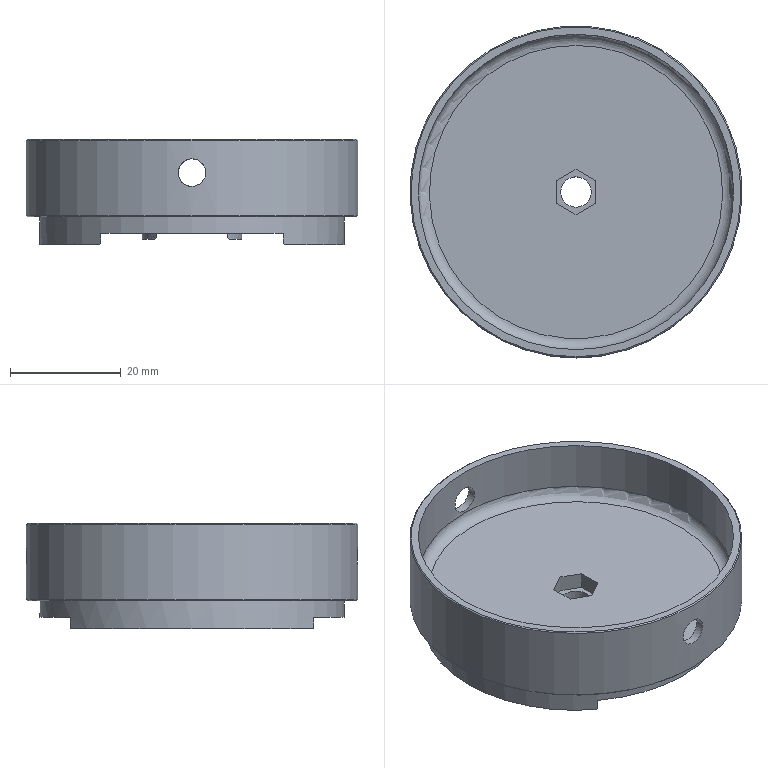NC program | NX | posted with a generic post | part box 60 x 60 x 19 mm
Lines 4673 to 5690 of 13134:
(ZLEVEL_PROFILE_COPY_1_COPY_COPY_COPY_COPY , TOOL : D2)
N9308 T23 M6
N9310 G54
N9312 G17 G0 G90 X-1.987 Y0.859 S5000 M3
N9314 G43 Z30. H23
N9316 Z-11.015
N9318 G94 G1 X-2.333 F1000.
N9320 G3 X-2.506 Y0.759 R0.2
N9322 G1 X-2.944 Y0.
N9324 X-2.506 Y-0.759
N9326 G3 X-2.333 Y-0.859 R0.2
N9328 G1 X-1.987
N9330 G0 Y0.859 Z-11.03
N9332 G1 X-2.333
N9334 G3 X-2.506 Y0.759 R0.2
N9336 G1 X-2.944 Y0.
N9338 X-2.506 Y-0.759
N9340 G3 X-2.333 Y-0.859 R0.2
N9342 G1 X-1.987
N9344 G0 Y0.859 Z-11.045
N9346 G1 X-2.333
N9348 G3 X-2.506 Y0.759 R0.2
N9350 G1 X-2.944 Y0.
N9352 X-2.506 Y-0.759
N9354 G3 X-2.333 Y-0.859 R0.2
N9356 G1 X-1.987
N9358 G0 Y0.859 Z-11.06
N9360 G1 X-2.333
N9362 G3 X-2.506 Y0.759 R0.2
N9364 G1 X-2.944 Y0.
N9366 X-2.506 Y-0.759
N9368 G3 X-2.333 Y-0.859 R0.2
N9370 G1 X-1.987
N9372 G0 Y0.859 Z-11.075
N9374 G1 X-2.333
N9376 G3 X-2.506 Y0.759 R0.2
N9378 G1 X-2.944 Y0.
N9380 X-2.506 Y-0.759
N9382 G3 X-2.333 Y-0.859 R0.2
N9384 G1 X-1.987
N9386 G0 Y0.859 Z-11.09
N9388 G1 X-2.333
N9390 G3 X-2.506 Y0.759 R0.2
N9392 G1 X-2.944 Y0.
N9394 X-2.506 Y-0.759
N9396 G3 X-2.333 Y-0.859 R0.2
N9398 G1 X-1.987
N9400 G0 Y0.859 Z-11.105
N9402 G1 X-2.333
N9404 G3 X-2.506 Y0.759 R0.2
N9406 G1 X-2.944 Y0.
N9408 X-2.506 Y-0.759
N9410 G3 X-2.333 Y-0.859 R0.2
N9412 G1 X-1.987
N9414 G0 Y0.859 Z-11.12
N9416 G1 X-2.333
N9418 G3 X-2.506 Y0.759 R0.2
N9420 G1 X-2.944 Y0.
N9422 X-2.506 Y-0.759
N9424 G3 X-2.333 Y-0.859 R0.2
N9426 G1 X-1.987
N9428 G0 Y0.859 Z-11.135
N9430 G1 X-2.333
N9432 G3 X-2.506 Y0.759 R0.2
N9434 G1 X-2.944 Y0.
N9436 X-2.506 Y-0.759
N9438 G3 X-2.333 Y-0.859 R0.2
N9440 G1 X-1.987
N9442 G0 Y0.859 Z-11.15
N9444 G1 X-2.333
N9446 G3 X-2.506 Y0.759 R0.2
N9448 G1 X-2.944 Y0.
N9450 X-2.506 Y-0.759
N9452 G3 X-2.333 Y-0.859 R0.2
N9454 G1 X-1.987
N9456 G0 Y0.859 Z-11.165
N9458 G1 X-2.333
N9460 G3 X-2.506 Y0.759 R0.2
N9462 G1 X-2.944 Y0.
N9464 X-2.506 Y-0.759
N9466 G3 X-2.333 Y-0.859 R0.2
N9468 G1 X-1.987
N9470 G0 Y0.859 Z-11.18
N9472 G1 X-2.333
N9474 G3 X-2.506 Y0.759 R0.2
N9476 G1 X-2.944 Y0.
N9478 X-2.506 Y-0.759
N9480 G3 X-2.333 Y-0.859 R0.2
N9482 G1 X-1.987
N9484 G0 Y0.859 Z-11.195
N9486 G1 X-2.333
N9488 G3 X-2.506 Y0.759 R0.2
N9490 G1 X-2.944 Y0.
N9492 X-2.506 Y-0.759
N9494 G3 X-2.333 Y-0.859 R0.2
N9496 G1 X-1.987
N9498 G0 Y0.859 Z-11.21
N9500 G1 X-2.333
N9502 G3 X-2.506 Y0.759 R0.2
N9504 G1 X-2.944 Y0.
N9506 X-2.506 Y-0.759
N9508 G3 X-2.333 Y-0.859 R0.2
N9510 G1 X-1.987
N9512 G0 Y0.859 Z-11.225
N9514 G1 X-2.333
N9516 G3 X-2.506 Y0.759 R0.2
N9518 G1 X-2.944 Y0.
N9520 X-2.506 Y-0.759
N9522 G3 X-2.333 Y-0.859 R0.2
N9524 G1 X-1.987
N9526 G0 Y0.859 Z-11.24
N9528 G1 X-2.333
N9530 G3 X-2.506 Y0.759 R0.2
N9532 G1 X-2.944 Y0.
N9534 X-2.506 Y-0.759
N9536 G3 X-2.333 Y-0.859 R0.2
N9538 G1 X-1.987
N9540 G0 Y0.859 Z-11.255
N9542 G1 X-2.333
N9544 G3 X-2.506 Y0.759 R0.2
N9546 G1 X-2.944 Y0.
N9548 X-2.506 Y-0.759
N9550 G3 X-2.333 Y-0.859 R0.2
N9552 G1 X-1.987
N9554 G0 Y0.859 Z-11.27
N9556 G1 X-2.333
N9558 G3 X-2.506 Y0.759 R0.2
N9560 G1 X-2.944 Y0.
N9562 X-2.506 Y-0.759
N9564 G3 X-2.333 Y-0.859 R0.2
N9566 G1 X-1.987
N9568 G0 Y0.859 Z-11.285
N9570 G1 X-2.333
N9572 G3 X-2.506 Y0.759 R0.2
N9574 G1 X-2.944 Y0.
N9576 X-2.506 Y-0.759
N9578 G3 X-2.333 Y-0.859 R0.2
N9580 G1 X-1.987
N9582 G0 Y0.859 Z-11.3
N9584 G1 X-2.333
N9586 G3 X-2.506 Y0.759 R0.2
N9588 G1 X-2.944 Y0.
N9590 X-2.506 Y-0.759
N9592 G3 X-2.333 Y-0.859 R0.2
N9594 G1 X-1.987
N9596 G0 Y0.859 Z-11.315
N9598 G1 X-2.333
N9600 G3 X-2.506 Y0.759 R0.2
N9602 G1 X-2.944 Y0.
N9604 X-2.506 Y-0.759
N9606 G3 X-2.333 Y-0.859 R0.2
N9608 G1 X-1.987
N9610 G0 Y0.859 Z-11.33
N9612 G1 X-2.333
N9614 G3 X-2.506 Y0.759 R0.2
N9616 G1 X-2.944 Y0.
N9618 X-2.506 Y-0.759
N9620 G3 X-2.333 Y-0.859 R0.2
N9622 G1 X-1.987
N9624 G0 Y0.859 Z-11.345
N9626 G1 X-2.333
N9628 G3 X-2.506 Y0.759 R0.2
N9630 G1 X-2.944 Y0.
N9632 X-2.506 Y-0.759
N9634 G3 X-2.333 Y-0.859 R0.2
N9636 G1 X-1.987
N9638 G0 Y0.859 Z-11.36
N9640 G1 X-2.333
N9642 G3 X-2.506 Y0.759 R0.2
N9644 G1 X-2.944 Y0.
N9646 X-2.506 Y-0.759
N9648 G3 X-2.333 Y-0.859 R0.2
N9650 G1 X-1.987
N9652 G0 Y0.859 Z-11.375
N9654 G1 X-2.333
N9656 G3 X-2.506 Y0.759 R0.2
N9658 G1 X-2.944 Y0.
N9660 X-2.506 Y-0.759
N9662 G3 X-2.333 Y-0.859 R0.2
N9664 G1 X-1.987
N9666 G0 Y0.859 Z-11.39
N9668 G1 X-2.333
N9670 G3 X-2.506 Y0.759 R0.2
N9672 G1 X-2.944 Y0.
N9674 X-2.506 Y-0.759
N9676 G3 X-2.333 Y-0.859 R0.2
N9678 G1 X-1.987
N9680 G0 Y0.859 Z-11.405
N9682 G1 X-2.333
N9684 G3 X-2.506 Y0.759 R0.2
N9686 G1 X-2.944 Y0.
N9688 X-2.506 Y-0.759
N9690 G3 X-2.333 Y-0.859 R0.2
N9692 G1 X-1.987
N9694 G0 Y0.859 Z-11.42
N9696 G1 X-2.333
N9698 G3 X-2.506 Y0.759 R0.2
N9700 G1 X-2.944 Y0.
N9702 X-2.506 Y-0.759
N9704 G3 X-2.333 Y-0.859 R0.2
N9706 G1 X-1.987
N9708 G0 Y0.859 Z-11.435
N9710 G1 X-2.333
N9712 G3 X-2.506 Y0.759 R0.2
N9714 G1 X-2.944 Y0.
N9716 X-2.506 Y-0.759
N9718 G3 X-2.333 Y-0.859 R0.2
N9720 G1 X-1.987
N9722 G0 Y0.859 Z-11.45
N9724 G1 X-2.333
N9726 G3 X-2.506 Y0.759 R0.2
N9728 G1 X-2.944 Y0.
N9730 X-2.506 Y-0.759
N9732 G3 X-2.333 Y-0.859 R0.2
N9734 G1 X-1.987
N9736 G0 Y0.859 Z-11.465
N9738 G1 X-2.333
N9740 G3 X-2.506 Y0.759 R0.2
N9742 G1 X-2.944 Y0.
N9744 X-2.506 Y-0.759
N9746 G3 X-2.333 Y-0.859 R0.2
N9748 G1 X-1.987
N9750 G0 Y0.859 Z-11.48
N9752 G1 X-2.333
N9754 G3 X-2.506 Y0.759 R0.2
N9756 G1 X-2.944 Y0.
N9758 X-2.506 Y-0.759
N9760 G3 X-2.333 Y-0.859 R0.2
N9762 G1 X-1.987
N9764 G0 Y0.859 Z-11.495
N9766 G1 X-2.333
N9768 G3 X-2.506 Y0.759 R0.2
N9770 G1 X-2.944 Y0.
N9772 X-2.506 Y-0.759
N9774 G3 X-2.333 Y-0.859 R0.2
N9776 G1 X-1.987
N9778 G0 Y0.859 Z-11.51
N9780 G1 X-2.333
N9782 G3 X-2.506 Y0.759 R0.2
N9784 G1 X-2.944 Y0.
N9786 X-2.506 Y-0.759
N9788 G3 X-2.333 Y-0.859 R0.2
N9790 G1 X-1.987
N9792 G0 Y0.859 Z-11.525
N9794 G1 X-2.333
N9796 G3 X-2.506 Y0.759 R0.2
N9798 G1 X-2.944 Y0.
N9800 X-2.506 Y-0.759
N9802 G3 X-2.333 Y-0.859 R0.2
N9804 G1 X-1.987
N9806 G0 Y0.859 Z-11.54
N9808 G1 X-2.333
N9810 G3 X-2.506 Y0.759 R0.2
N9812 G1 X-2.944 Y0.
N9814 X-2.506 Y-0.759
N9816 G3 X-2.333 Y-0.859 R0.2
N9818 G1 X-1.987
N9820 G0 Y0.859 Z-11.555
N9822 G1 X-2.333
N9824 G3 X-2.506 Y0.759 R0.2
N9826 G1 X-2.944 Y0.
N9828 X-2.506 Y-0.759
N9830 G3 X-2.333 Y-0.859 R0.2
N9832 G1 X-1.987
N9834 G0 Y0.859 Z-11.57
N9836 G1 X-2.333
N9838 G3 X-2.506 Y0.759 R0.2
N9840 G1 X-2.944 Y0.
N9842 X-2.506 Y-0.759
N9844 G3 X-2.333 Y-0.859 R0.2
N9846 G1 X-1.987
N9848 G0 Y0.859 Z-11.585
N9850 G1 X-2.333
N9852 G3 X-2.506 Y0.759 R0.2
N9854 G1 X-2.944 Y0.
N9856 X-2.506 Y-0.759
N9858 G3 X-2.333 Y-0.859 R0.2
N9860 G1 X-1.987
N9862 G0 Y0.859 Z-11.6
N9864 G1 X-2.333
N9866 G3 X-2.506 Y0.759 R0.2
N9868 G1 X-2.944 Y0.
N9870 X-2.506 Y-0.759
N9872 G3 X-2.333 Y-0.859 R0.2
N9874 G1 X-1.987
N9876 G0 Y0.859 Z-11.615
N9878 G1 X-2.333
N9880 G3 X-2.506 Y0.759 R0.2
N9882 G1 X-2.944 Y0.
N9884 X-2.506 Y-0.759
N9886 G3 X-2.333 Y-0.859 R0.2
N9888 G1 X-1.987
N9890 G0 Y0.859 Z-11.63
N9892 G1 X-2.333
N9894 G3 X-2.506 Y0.759 R0.2
N9896 G1 X-2.944 Y0.
N9898 X-2.506 Y-0.759
N9900 G3 X-2.333 Y-0.859 R0.2
N9902 G1 X-1.987
N9904 G0 Y0.859 Z-11.645
N9906 G1 X-2.333
N9908 G3 X-2.506 Y0.759 R0.2
N9910 G1 X-2.944 Y0.
N9912 X-2.506 Y-0.759
N9914 G3 X-2.333 Y-0.859 R0.2
N9916 G1 X-1.987
N9918 G0 Y0.859 Z-11.66
N9920 G1 X-2.333
N9922 G3 X-2.506 Y0.759 R0.2
N9924 G1 X-2.944 Y0.
N9926 X-2.506 Y-0.759
N9928 G3 X-2.333 Y-0.859 R0.2
N9930 G1 X-1.987
N9932 G0 Y0.859 Z-11.675
N9934 G1 X-2.333
N9936 G3 X-2.506 Y0.759 R0.2
N9938 G1 X-2.944 Y0.
N9940 X-2.506 Y-0.759
N9942 G3 X-2.333 Y-0.859 R0.2
N9944 G1 X-1.987
N9946 G0 Y0.859 Z-11.69
N9948 G1 X-2.333
N9950 G3 X-2.506 Y0.759 R0.2
N9952 G1 X-2.944 Y0.
N9954 X-2.506 Y-0.759
N9956 G3 X-2.333 Y-0.859 R0.2
N9958 G1 X-1.987
N9960 G0 Y0.859 Z-11.705
N9962 G1 X-2.333
N9964 G3 X-2.506 Y0.759 R0.2
N9966 G1 X-2.944 Y0.
N9968 X-2.506 Y-0.759
N9970 G3 X-2.333 Y-0.859 R0.2
N9972 G1 X-1.987
N9974 G0 Y0.859 Z-11.72
N9976 G1 X-2.333
N9978 G3 X-2.506 Y0.759 R0.2
N9980 G1 X-2.944 Y0.
N9982 X-2.506 Y-0.759
N9984 G3 X-2.333 Y-0.859 R0.2
N9986 G1 X-1.987
N9988 G0 Y0.859 Z-11.735
N9990 G1 X-2.333
N9992 G3 X-2.506 Y0.759 R0.2
N9994 G1 X-2.944 Y0.
N9996 X-2.506 Y-0.759
N9998 G3 X-2.333 Y-0.859 R0.2
N10000 G1 X-1.987
N10002 G0 Y0.859 Z-11.75
N10004 G1 X-2.333
N10006 G3 X-2.506 Y0.759 R0.2
N10008 G1 X-2.944 Y0.
N10010 X-2.506 Y-0.759
N10012 G3 X-2.333 Y-0.859 R0.2
N10014 G1 X-1.987
N10016 G0 Y0.859 Z-11.765
N10018 G1 X-2.333
N10020 G3 X-2.506 Y0.759 R0.2
N10022 G1 X-2.944 Y0.
N10024 X-2.506 Y-0.759
N10026 G3 X-2.333 Y-0.859 R0.2
N10028 G1 X-1.987
N10030 G0 Y0.859 Z-11.78
N10032 G1 X-2.333
N10034 G3 X-2.506 Y0.759 R0.2
N10036 G1 X-2.944 Y0.
N10038 X-2.506 Y-0.759
N10040 G3 X-2.333 Y-0.859 R0.2
N10042 G1 X-1.987
N10044 G0 Y0.859 Z-11.795
N10046 G1 X-2.333
N10048 G3 X-2.506 Y0.759 R0.2
N10050 G1 X-2.944 Y0.
N10052 X-2.506 Y-0.759
N10054 G3 X-2.333 Y-0.859 R0.2
N10056 G1 X-1.987
N10058 G0 Y0.859 Z-11.81
N10060 G1 X-2.333
N10062 G3 X-2.506 Y0.759 R0.2
N10064 G1 X-2.944 Y0.
N10066 X-2.506 Y-0.759
N10068 G3 X-2.333 Y-0.859 R0.2
N10070 G1 X-1.987
N10072 G0 Y0.859 Z-11.825
N10074 G1 X-2.333
N10076 G3 X-2.506 Y0.759 R0.2
N10078 G1 X-2.944 Y0.
N10080 X-2.506 Y-0.759
N10082 G3 X-2.333 Y-0.859 R0.2
N10084 G1 X-1.987
N10086 G0 Y0.859 Z-11.84
N10088 G1 X-2.333
N10090 G3 X-2.506 Y0.759 R0.2
N10092 G1 X-2.944 Y0.
N10094 X-2.506 Y-0.759
N10096 G3 X-2.333 Y-0.859 R0.2
N10098 G1 X-1.987
N10100 G0 Y0.859 Z-11.855
N10102 G1 X-2.333
N10104 G3 X-2.506 Y0.759 R0.2
N10106 G1 X-2.944 Y0.
N10108 X-2.506 Y-0.759
N10110 G3 X-2.333 Y-0.859 R0.2
N10112 G1 X-1.987
N10114 G0 Y0.859 Z-11.87
N10116 G1 X-2.333
N10118 G3 X-2.506 Y0.759 R0.2
N10120 G1 X-2.944 Y0.
N10122 X-2.506 Y-0.759
N10124 G3 X-2.333 Y-0.859 R0.2
N10126 G1 X-1.987
N10128 G0 Y0.859 Z-11.885
N10130 G1 X-2.333
N10132 G3 X-2.506 Y0.759 R0.2
N10134 G1 X-2.944 Y0.
N10136 X-2.506 Y-0.759
N10138 G3 X-2.333 Y-0.859 R0.2
N10140 G1 X-1.987
N10142 G0 Y0.859 Z-11.9
N10144 G1 X-2.333
N10146 G3 X-2.506 Y0.759 R0.2
N10148 G1 X-2.944 Y0.
N10150 X-2.506 Y-0.759
N10152 G3 X-2.333 Y-0.859 R0.2
N10154 G1 X-1.987
N10156 G0 Y0.859 Z-11.915
N10158 G1 X-2.333
N10160 G3 X-2.506 Y0.759 R0.2
N10162 G1 X-2.944 Y0.
N10164 X-2.506 Y-0.759
N10166 G3 X-2.333 Y-0.859 R0.2
N10168 G1 X-1.987
N10170 G0 Y0.859 Z-11.93
N10172 G1 X-2.333
N10174 G3 X-2.506 Y0.759 R0.2
N10176 G1 X-2.944 Y0.
N10178 X-2.506 Y-0.759
N10180 G3 X-2.333 Y-0.859 R0.2
N10182 G1 X-1.987
N10184 G0 Y0.859 Z-11.945
N10186 G1 X-2.333
N10188 G3 X-2.506 Y0.759 R0.2
N10190 G1 X-2.944 Y0.
N10192 X-2.506 Y-0.759
N10194 G3 X-2.333 Y-0.859 R0.2
N10196 G1 X-1.987
N10198 G0 Y0.859 Z-11.96
N10200 G1 X-2.333
N10202 G3 X-2.506 Y0.759 R0.2
N10204 G1 X-2.944 Y0.
N10206 X-2.506 Y-0.759
N10208 G3 X-2.333 Y-0.859 R0.2
N10210 G1 X-1.987
N10212 G0 Y0.859 Z-11.975
N10214 G1 X-2.333
N10216 G3 X-2.506 Y0.759 R0.2
N10218 G1 X-2.944 Y0.
N10220 X-2.506 Y-0.759
N10222 G3 X-2.333 Y-0.859 R0.2
N10224 G1 X-1.987
N10226 G0 Y0.859 Z-11.99
N10228 G1 X-2.333
N10230 G3 X-2.506 Y0.759 R0.2
N10232 G1 X-2.944 Y0.
N10234 X-2.506 Y-0.759
N10236 G3 X-2.333 Y-0.859 R0.2
N10238 G1 X-1.987
N10240 G0 Y0.859 Z-12.005
N10242 G1 X-2.333
N10244 G3 X-2.506 Y0.759 R0.2
N10246 G1 X-2.944 Y0.
N10248 X-2.506 Y-0.759
N10250 G3 X-2.333 Y-0.859 R0.2
N10252 G1 X-1.987
N10254 G0 Y0.859 Z-12.02
N10256 G1 X-2.333
N10258 G3 X-2.506 Y0.759 R0.2
N10260 G1 X-2.944 Y0.
N10262 X-2.506 Y-0.759
N10264 G3 X-2.333 Y-0.859 R0.2
N10266 G1 X-1.987
N10268 G0 Y0.859 Z-12.035
N10270 G1 X-2.333
N10272 G3 X-2.506 Y0.759 R0.2
N10274 G1 X-2.944 Y0.
N10276 X-2.506 Y-0.759
N10278 G3 X-2.333 Y-0.859 R0.2
N10280 G1 X-1.987
N10282 G0 Y0.859 Z-12.05
N10284 G1 X-2.333
N10286 G3 X-2.506 Y0.759 R0.2
N10288 G1 X-2.944 Y0.
N10290 X-2.506 Y-0.759
N10292 G3 X-2.333 Y-0.859 R0.2
N10294 G1 X-1.987
N10296 G0 Y0.859 Z-12.065
N10298 G1 X-2.333
N10300 G3 X-2.506 Y0.759 R0.2
N10302 G1 X-2.944 Y0.
N10304 X-2.506 Y-0.759
N10306 G3 X-2.333 Y-0.859 R0.2
N10308 G1 X-1.987
N10310 G0 Y0.859 Z-12.08
N10312 G1 X-2.333
N10314 G3 X-2.506 Y0.759 R0.2
N10316 G1 X-2.944 Y0.
N10318 X-2.506 Y-0.759
N10320 G3 X-2.333 Y-0.859 R0.2
N10322 G1 X-1.987
N10324 G0 Y0.859 Z-12.095
N10326 G1 X-2.333
N10328 G3 X-2.506 Y0.759 R0.2
N10330 G1 X-2.944 Y0.
N10332 X-2.506 Y-0.759
N10334 G3 X-2.333 Y-0.859 R0.2
N10336 G1 X-1.987
N10338 G0 Y0.859 Z-12.11
N10340 G1 X-2.333
N10342 G3 X-2.506 Y0.759 R0.2
N10344 G1 X-2.944 Y0.
N10346 X-2.506 Y-0.759
N10348 G3 X-2.333 Y-0.859 R0.2
N10350 G1 X-1.987
N10352 G0 Y0.859 Z-12.125
N10354 G1 X-2.333
N10356 G3 X-2.506 Y0.759 R0.2
N10358 G1 X-2.944 Y0.
N10360 X-2.506 Y-0.759
N10362 G3 X-2.333 Y-0.859 R0.2
N10364 G1 X-1.987
N10366 G0 Y0.859 Z-12.14
N10368 G1 X-2.333
N10370 G3 X-2.506 Y0.759 R0.2
N10372 G1 X-2.944 Y0.
N10374 X-2.506 Y-0.759
N10376 G3 X-2.333 Y-0.859 R0.2
N10378 G1 X-1.987
N10380 G0 Y0.859 Z-12.155
N10382 G1 X-2.333
N10384 G3 X-2.506 Y0.759 R0.2
N10386 G1 X-2.944 Y0.
N10388 X-2.506 Y-0.759
N10390 G3 X-2.333 Y-0.859 R0.2
N10392 G1 X-1.987
N10394 G0 Y0.859 Z-12.17
N10396 G1 X-2.333
N10398 G3 X-2.506 Y0.759 R0.2
N10400 G1 X-2.944 Y0.
N10402 X-2.506 Y-0.759
N10404 G3 X-2.333 Y-0.859 R0.2
N10406 G1 X-1.987
N10408 G0 Y0.859 Z-12.185
N10410 G1 X-2.333
N10412 G3 X-2.506 Y0.759 R0.2
N10414 G1 X-2.944 Y0.
N10416 X-2.506 Y-0.759
N10418 G3 X-2.333 Y-0.859 R0.2
N10420 G1 X-1.987
N10422 G0 Y0.859 Z-12.2
N10424 G1 X-2.333
N10426 G3 X-2.506 Y0.759 R0.2
N10428 G1 X-2.944 Y0.
N10430 X-2.506 Y-0.759
N10432 G3 X-2.333 Y-0.859 R0.2
N10434 G1 X-1.987
N10436 G0 Y0.859 Z-12.215
N10438 G1 X-2.333
N10440 G3 X-2.506 Y0.759 R0.2
N10442 G1 X-2.944 Y0.
N10444 X-2.506 Y-0.759
N10446 G3 X-2.333 Y-0.859 R0.2
N10448 G1 X-1.987
N10450 G0 Y0.859 Z-12.23
N10452 G1 X-2.333
N10454 G3 X-2.506 Y0.759 R0.2
N10456 G1 X-2.944 Y0.
N10458 X-2.506 Y-0.759
N10460 G3 X-2.333 Y-0.859 R0.2
N10462 G1 X-1.987
N10464 G0 Y0.859 Z-12.245
N10466 G1 X-2.333
N10468 G3 X-2.506 Y0.759 R0.2
N10470 G1 X-2.944 Y0.
N10472 X-2.506 Y-0.759
N10474 G3 X-2.333 Y-0.859 R0.2
N10476 G1 X-1.987
N10478 G0 Y0.859 Z-12.26
N10480 G1 X-2.333
N10482 G3 X-2.506 Y0.759 R0.2
N10484 G1 X-2.944 Y0.
N10486 X-2.506 Y-0.759
N10488 G3 X-2.333 Y-0.859 R0.2
N10490 G1 X-1.987
N10492 G0 Y0.859 Z-12.275
N10494 G1 X-2.333
N10496 G3 X-2.506 Y0.759 R0.2
N10498 G1 X-2.944 Y0.
N10500 X-2.506 Y-0.759
N10502 G3 X-2.333 Y-0.859 R0.2
N10504 G1 X-1.987
N10506 G0 Y0.859 Z-12.29
N10508 G1 X-2.333
N10510 G3 X-2.506 Y0.759 R0.2
N10512 G1 X-2.944 Y0.
N10514 X-2.506 Y-0.759
N10516 G3 X-2.333 Y-0.859 R0.2
N10518 G1 X-1.987
N10520 G0 Y0.859 Z-12.305
N10522 G1 X-2.333
N10524 G3 X-2.506 Y0.759 R0.2
N10526 G1 X-2.944 Y0.
N10528 X-2.506 Y-0.759
N10530 G3 X-2.333 Y-0.859 R0.2
N10532 G1 X-1.987
N10534 G0 Y0.859 Z-12.32
N10536 G1 X-2.333
N10538 G3 X-2.506 Y0.759 R0.2
N10540 G1 X-2.944 Y0.
N10542 X-2.506 Y-0.759
N10544 G3 X-2.333 Y-0.859 R0.2
N10546 G1 X-1.987
N10548 G0 Y0.859 Z-12.335
N10550 G1 X-2.333
N10552 G3 X-2.506 Y0.759 R0.2
N10554 G1 X-2.944 Y0.
N10556 X-2.506 Y-0.759
N10558 G3 X-2.333 Y-0.859 R0.2
N10560 G1 X-1.987
N10562 G0 Y0.859 Z-12.35
N10564 G1 X-2.333
N10566 G3 X-2.506 Y0.759 R0.2
N10568 G1 X-2.944 Y0.
N10570 X-2.506 Y-0.759
N10572 G3 X-2.333 Y-0.859 R0.2
N10574 G1 X-1.987
N10576 G0 Y0.859 Z-12.365
N10578 G1 X-2.333
N10580 G3 X-2.506 Y0.759 R0.2
N10582 G1 X-2.944 Y0.
N10584 X-2.506 Y-0.759
N10586 G3 X-2.333 Y-0.859 R0.2
N10588 G1 X-1.987
N10590 G0 Y0.859 Z-12.38
N10592 G1 X-2.333
N10594 G3 X-2.506 Y0.759 R0.2
N10596 G1 X-2.944 Y0.
N10598 X-2.506 Y-0.759
N10600 G3 X-2.333 Y-0.859 R0.2
N10602 G1 X-1.987
N10604 G0 Y0.859 Z-12.395
N10606 G1 X-2.333
N10608 G3 X-2.506 Y0.759 R0.2
N10610 G1 X-2.944 Y0.
N10612 X-2.506 Y-0.759
N10614 G3 X-2.333 Y-0.859 R0.2
N10616 G1 X-1.987
N10618 G0 Y0.859 Z-12.41
N10620 G1 X-2.333
N10622 G3 X-2.506 Y0.759 R0.2
N10624 G1 X-2.944 Y0.
N10626 X-2.506 Y-0.759
N10628 G3 X-2.333 Y-0.859 R0.2
N10630 G1 X-1.987
N10632 G0 Y0.859 Z-12.425
N10634 G1 X-2.333
N10636 G3 X-2.506 Y0.759 R0.2
N10638 G1 X-2.944 Y0.
N10640 X-2.506 Y-0.759
N10642 G3 X-2.333 Y-0.859 R0.2
N10644 G1 X-1.987
N10646 G0 Y0.859 Z-12.44
N10648 G1 X-2.333
N10650 G3 X-2.506 Y0.759 R0.2
N10652 G1 X-2.944 Y0.
N10654 X-2.506 Y-0.759
N10656 G3 X-2.333 Y-0.859 R0.2
N10658 G1 X-1.987
N10660 G0 Y0.859 Z-12.455
N10662 G1 X-2.333
N10664 G3 X-2.506 Y0.759 R0.2
N10666 G1 X-2.944 Y0.
N10668 X-2.506 Y-0.759
N10670 G3 X-2.333 Y-0.859 R0.2
N10672 G1 X-1.987
N10674 G0 Y0.859 Z-12.47
N10676 G1 X-2.333
N10678 G3 X-2.506 Y0.759 R0.2
N10680 G1 X-2.944 Y0.
N10682 X-2.506 Y-0.759
N10684 G3 X-2.333 Y-0.859 R0.2
N10686 G1 X-1.987
N10688 G0 Y0.859 Z-12.485
N10690 G1 X-2.333
N10692 G3 X-2.506 Y0.759 R0.2
N10694 G1 X-2.944 Y0.
N10696 X-2.506 Y-0.759
N10698 G3 X-2.333 Y-0.859 R0.2
N10700 G1 X-1.987
N10702 G0 Y0.859 Z-12.5
N10704 G1 X-2.333
N10706 G3 X-2.506 Y0.759 R0.2
N10708 G1 X-2.944 Y0.
N10710 X-2.506 Y-0.759
N10712 G3 X-2.333 Y-0.859 R0.2
N10714 G1 X-1.987
N10716 G0 Y0.859 Z-12.515
N10718 G1 X-2.333
N10720 G3 X-2.506 Y0.759 R0.2
N10722 G1 X-2.944 Y0.
N10724 X-2.506 Y-0.759
N10726 G3 X-2.333 Y-0.859 R0.2
N10728 G1 X-1.987
N10730 G0 Y0.859 Z-12.53
N10732 G1 X-2.333
N10734 G3 X-2.506 Y0.759 R0.2
N10736 G1 X-2.944 Y0.
N10738 X-2.506 Y-0.759
N10740 G3 X-2.333 Y-0.859 R0.2
N10742 G1 X-1.987
N10744 G0 Y0.859 Z-12.545
N10746 G1 X-2.333
N10748 G3 X-2.506 Y0.759 R0.2
N10750 G1 X-2.944 Y0.
N10752 X-2.506 Y-0.759
N10754 G3 X-2.333 Y-0.859 R0.2
N10756 G1 X-1.987
N10758 G0 Y0.859 Z-12.56
N10760 G1 X-2.333
N10762 G3 X-2.506 Y0.759 R0.2
N10764 G1 X-2.944 Y0.
N10766 X-2.506 Y-0.759
N10768 G3 X-2.333 Y-0.859 R0.2
N10770 G1 X-1.987
N10772 G0 Y0.859 Z-12.575
N10774 G1 X-2.333
N10776 G3 X-2.506 Y0.759 R0.2
N10778 G1 X-2.944 Y0.
N10780 X-2.506 Y-0.759
N10782 G3 X-2.333 Y-0.859 R0.2
N10784 G1 X-1.987
N10786 G0 Y0.859 Z-12.59
N10788 G1 X-2.333
N10790 G3 X-2.506 Y0.759 R0.2
N10792 G1 X-2.944 Y0.
N10794 X-2.506 Y-0.759
N10796 G3 X-2.333 Y-0.859 R0.2
N10798 G1 X-1.987
N10800 G0 Y0.859 Z-12.605
N10802 G1 X-2.333
N10804 G3 X-2.506 Y0.759 R0.2
N10806 G1 X-2.944 Y0.
N10808 X-2.506 Y-0.759
N10810 G3 X-2.333 Y-0.859 R0.2
N10812 G1 X-1.987
N10814 G0 Y0.859 Z-12.62
N10816 G1 X-2.333
N10818 G3 X-2.506 Y0.759 R0.2
N10820 G1 X-2.944 Y0.
N10822 X-2.506 Y-0.759
N10824 G3 X-2.333 Y-0.859 R0.2
N10826 G1 X-1.987
N10828 G0 Y0.859 Z-12.635
N10830 G1 X-2.333
N10832 G3 X-2.506 Y0.759 R0.2
N10834 G1 X-2.944 Y0.
N10836 X-2.506 Y-0.759
N10838 G3 X-2.333 Y-0.859 R0.2
N10840 G1 X-1.987
N10842 G0 Y0.859 Z-12.65
N10844 G1 X-2.333
N10846 G3 X-2.506 Y0.759 R0.2
N10848 G1 X-2.944 Y0.
N10850 X-2.506 Y-0.759
N10852 G3 X-2.333 Y-0.859 R0.2
N10854 G1 X-1.987
N10856 G0 Y0.859 Z-12.665
N10858 G1 X-2.333
N10860 G3 X-2.506 Y0.759 R0.2
N10862 G1 X-2.944 Y0.
N10864 X-2.506 Y-0.759
N10866 G3 X-2.333 Y-0.859 R0.2
N10868 G1 X-1.987
N10870 G0 Y0.859 Z-12.68
N10872 G1 X-2.333
N10874 G3 X-2.506 Y0.759 R0.2
N10876 G1 X-2.944 Y0.
N10878 X-2.506 Y-0.759
N10880 G3 X-2.333 Y-0.859 R0.2
N10882 G1 X-1.987
N10884 G0 Y0.859 Z-12.695
N10886 G1 X-2.333
N10888 G3 X-2.506 Y0.759 R0.2
N10890 G1 X-2.944 Y0.
N10892 X-2.506 Y-0.759
N10894 G3 X-2.333 Y-0.859 R0.2
N10896 G1 X-1.987
N10898 G0 Y0.859 Z-12.71
N10900 G1 X-2.333
N10902 G3 X-2.506 Y0.759 R0.2
N10904 G1 X-2.944 Y0.
N10906 X-2.506 Y-0.759
N10908 G3 X-2.333 Y-0.859 R0.2
N10910 G1 X-1.987
N10912 G0 Y0.859 Z-12.725
N10914 G1 X-2.333
N10916 G3 X-2.506 Y0.759 R0.2
N10918 G1 X-2.944 Y0.
N10920 X-2.506 Y-0.759
N10922 G3 X-2.333 Y-0.859 R0.2
N10924 G1 X-1.987
N10926 G0 Y0.859 Z-12.74
N10928 G1 X-2.333
N10930 G3 X-2.506 Y0.759 R0.2
N10932 G1 X-2.944 Y0.
N10934 X-2.506 Y-0.759
N10936 G3 X-2.333 Y-0.859 R0.2
N10938 G1 X-1.987
N10940 G0 Y0.859 Z-12.755
N10942 G1 X-2.333
N10944 G3 X-2.506 Y0.759 R0.2
N10946 G1 X-2.944 Y0.
N10948 X-2.506 Y-0.759
N10950 G3 X-2.333 Y-0.859 R0.2
N10952 G1 X-1.987
N10954 G0 Y0.859 Z-12.77
N10956 G1 X-2.333
N10958 G3 X-2.506 Y0.759 R0.2
N10960 G1 X-2.944 Y0.
N10962 X-2.506 Y-0.759
N10964 G3 X-2.333 Y-0.859 R0.2
N10966 G1 X-1.987
N10968 G0 Y0.859 Z-12.785
N10970 G1 X-2.333
N10972 G3 X-2.506 Y0.759 R0.2
N10974 G1 X-2.944 Y0.
N10976 X-2.506 Y-0.759
N10978 G3 X-2.333 Y-0.859 R0.2
N10980 G1 X-1.987
N10982 G0 Y0.859 Z-12.8
N10984 G1 X-2.333
N10986 G3 X-2.506 Y0.759 R0.2
N10988 G1 X-2.944 Y0.
N10990 X-2.506 Y-0.759
N10992 G3 X-2.333 Y-0.859 R0.2
N10994 G1 X-1.987
N10996 G0 Y0.859 Z-12.815
N10998 G1 X-2.333
N11000 G3 X-2.506 Y0.759 R0.2
N11002 G1 X-2.944 Y0.
N11004 X-2.506 Y-0.759
N11006 G3 X-2.333 Y-0.859 R0.2
N11008 G1 X-1.987
N11010 G0 Y0.859 Z-12.83
N11012 G1 X-2.333
N11014 G3 X-2.506 Y0.759 R0.2
N11016 G1 X-2.944 Y0.
N11018 X-2.506 Y-0.759
N11020 G3 X-2.333 Y-0.859 R0.2
N11022 G1 X-1.987
N11024 G0 Y0.859 Z-12.845
N11026 G1 X-2.333
N11028 G3 X-2.506 Y0.759 R0.2
N11030 G1 X-2.944 Y0.
N11032 X-2.506 Y-0.759
N11034 G3 X-2.333 Y-0.859 R0.2
N11036 G1 X-1.987
N11038 G0 Y0.859 Z-12.86
N11040 G1 X-2.333
N11042 G3 X-2.506 Y0.759 R0.2
N11044 G1 X-2.944 Y0.
N11046 X-2.506 Y-0.759
N11048 G3 X-2.333 Y-0.859 R0.2
N11050 G1 X-1.987
N11052 G0 Y0.859 Z-12.875
N11054 G1 X-2.333
N11056 G3 X-2.506 Y0.759 R0.2
N11058 G1 X-2.944 Y0.
N11060 X-2.506 Y-0.759
N11062 G3 X-2.333 Y-0.859 R0.2
N11064 G1 X-1.987
N11066 G0 Y0.859 Z-12.89
N11068 G1 X-2.333
N11070 G3 X-2.506 Y0.759 R0.2
N11072 G1 X-2.944 Y0.
N11074 X-2.506 Y-0.759
N11076 G3 X-2.333 Y-0.859 R0.2
N11078 G1 X-1.987
N11080 G0 Y0.859 Z-12.905
N11082 G1 X-2.333
N11084 G3 X-2.506 Y0.759 R0.2
N11086 G1 X-2.944 Y0.
N11088 X-2.506 Y-0.759
N11090 G3 X-2.333 Y-0.859 R0.2
N11092 G1 X-1.987
N11094 G0 Y0.859 Z-12.92
N11096 G1 X-2.333
N11098 G3 X-2.506 Y0.759 R0.2
N11100 G1 X-2.944 Y0.
N11102 X-2.506 Y-0.759
N11104 G3 X-2.333 Y-0.859 R0.2
N11106 G1 X-1.987
N11108 G0 Y0.859 Z-12.935
N11110 G1 X-2.333
N11112 G3 X-2.506 Y0.759 R0.2
N11114 G1 X-2.944 Y0.
N11116 X-2.506 Y-0.759
N11118 G3 X-2.333 Y-0.859 R0.2
N11120 G1 X-1.987
N11122 G0 Y0.859 Z-12.95
N11124 G1 X-2.333
N11126 G3 X-2.506 Y0.759 R0.2
N11128 G1 X-2.944 Y0.
N11130 X-2.506 Y-0.759
N11132 G3 X-2.333 Y-0.859 R0.2
N11134 G1 X-1.987
N11136 G0 Y0.859 Z-12.965
N11138 G1 X-2.333
N11140 G3 X-2.506 Y0.759 R0.2
N11142 G1 X-2.944 Y0.
N11144 X-2.506 Y-0.759
N11146 G3 X-2.333 Y-0.859 R0.2
N11148 G1 X-1.987
N11150 G0 Y0.859 Z-12.98
N11152 G1 X-2.333
N11154 G3 X-2.506 Y0.759 R0.2
N11156 G1 X-2.944 Y0.
N11158 X-2.506 Y-0.759
N11160 G3 X-2.333 Y-0.859 R0.2
N11162 G1 X-1.987
N11164 G0 Y0.859 Z-12.995
N11166 G1 X-2.333
N11168 G3 X-2.506 Y0.759 R0.2
N11170 G1 X-2.944 Y0.
N11172 X-2.506 Y-0.759
N11174 G3 X-2.333 Y-0.859 R0.2
N11176 G1 X-1.987
N11178 G0 Y0.859 Z-13.01
N11180 G1 X-2.333
N11182 G3 X-2.506 Y0.759 R0.2
N11184 G1 X-2.944 Y0.
N11186 X-2.506 Y-0.759
N11188 G3 X-2.333 Y-0.859 R0.2
N11190 G1 X-1.987
N11192 G0 Y0.859 Z-13.025
N11194 G1 X-2.333
N11196 G3 X-2.506 Y0.759 R0.2
N11198 G1 X-2.944 Y0.
N11200 X-2.506 Y-0.759
N11202 G3 X-2.333 Y-0.859 R0.2
N11204 G1 X-1.987
N11206 G0 Y0.859 Z-13.04
N11208 G1 X-2.333
N11210 G3 X-2.506 Y0.759 R0.2
N11212 G1 X-2.944 Y0.
N11214 X-2.506 Y-0.759
N11216 G3 X-2.333 Y-0.859 R0.2
N11218 G1 X-1.987
N11220 G0 Y0.859 Z-13.055
N11222 G1 X-2.333
N11224 G3 X-2.506 Y0.759 R0.2
N11226 G1 X-2.944 Y0.
N11228 X-2.506 Y-0.759
N11230 G3 X-2.333 Y-0.859 R0.2
N11232 G1 X-1.987
N11234 G0 Y0.859 Z-13.07
N11236 G1 X-2.333
N11238 G3 X-2.506 Y0.759 R0.2
N11240 G1 X-2.944 Y0.
N11242 X-2.506 Y-0.759
N11244 G3 X-2.333 Y-0.859 R0.2
N11246 G1 X-1.987
N11248 G0 Y0.859 Z-13.085
N11250 G1 X-2.333
N11252 G3 X-2.506 Y0.759 R0.2
N11254 G1 X-2.944 Y0.
N11256 X-2.506 Y-0.759
N11258 G3 X-2.333 Y-0.859 R0.2
N11260 G1 X-1.987
N11262 G0 Y0.859 Z-13.1
N11264 G1 X-2.333
N11266 G3 X-2.506 Y0.759 R0.2
N11268 G1 X-2.944 Y0.
N11270 X-2.506 Y-0.759
N11272 G3 X-2.333 Y-0.859 R0.2
N11274 G1 X-1.987
N11276 G0 Y0.859 Z-13.115
N11278 G1 X-2.333
N11280 G3 X-2.506 Y0.759 R0.2
N11282 G1 X-2.944 Y0.
N11284 X-2.506 Y-0.759
N11286 G3 X-2.333 Y-0.859 R0.2
N11288 G1 X-1.987
N11290 G0 Y0.859 Z-13.13
N11292 G1 X-2.333
N11294 G3 X-2.506 Y0.759 R0.2
N11296 G1 X-2.944 Y0.
N11298 X-2.506 Y-0.759
N11300 G3 X-2.333 Y-0.859 R0.2
N11302 G1 X-1.987
N11304 G0 Y0.859 Z-13.145
N11306 G1 X-2.333
N11308 G3 X-2.506 Y0.759 R0.2
N11310 G1 X-2.944 Y0.
N11312 X-2.506 Y-0.759
N11314 G3 X-2.333 Y-0.859 R0.2
N11316 G1 X-1.987
N11318 G0 Y0.859 Z-13.16
N11320 G1 X-2.333
N11322 G3 X-2.506 Y0.759 R0.2
N11324 G1 X-2.944 Y0.
N11326 X-2.506 Y-0.759
N11328 G3 X-2.333 Y-0.859 R0.2
N11330 G1 X-1.987
N11332 G0 Y0.859 Z-13.175
N11334 G1 X-2.333
N11336 G3 X-2.506 Y0.759 R0.2